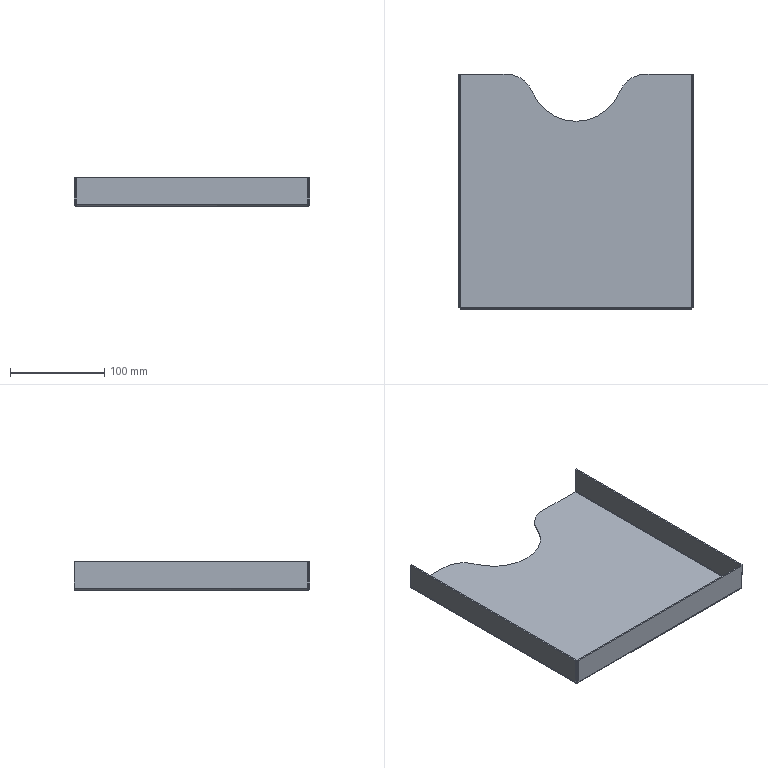Part | SolidWorks | features EdgeFlange 1, Fillet 1, FlatPattern 1, ICE 1, SMBaseFlange 1, SheetMetal 1 | 1 solid | 34 faces | box 250 x 250 x 30 mm | volume 118526 mm3 | plane 21 | cylinder 9 | spline 4 | commonest cylinder face diameters 1.473 x3 4.473 x3 60 x2 100 x1
STEP:
#1=CARTESIAN_POINT('',(122.763,125.,-1.5));
#2=VERTEX_POINT('',#1);
#3=CARTESIAN_POINT('',(74.162,125.,-1.5));
#4=VERTEX_POINT('',#3);
#5=CARTESIAN_POINT('',(-125.,125.,-1.5));
#6=DIRECTION('',(-1.,0.,0.));
#7=VECTOR('',#6,1000.);
#8=LINE('',#5,#7);
#9=EDGE_CURVE('',#2,#4,#8,.T.);
#10=ORIENTED_EDGE('',*,*,#9,.T.);
#11=CARTESIAN_POINT('',(74.162,125.,0.));
#12=VERTEX_POINT('',#11);
#13=CARTESIAN_POINT('',(74.162,125.,0.));
#14=DIRECTION('',(0.,0.,1.));
#15=VECTOR('',#14,1000.);
#16=LINE('',#13,#15);
#17=EDGE_CURVE('',#4,#12,#16,.T.);
#18=ORIENTED_EDGE('',*,*,#17,.T.);
#19=CARTESIAN_POINT('',(122.763,125.,0.));
#20=VERTEX_POINT('',#19);
#21=CARTESIAN_POINT('',(-125.,125.,0.));
#22=DIRECTION('',(-1.,0.,0.));
#23=VECTOR('',#22,1000.);
#24=LINE('',#21,#23);
#25=EDGE_CURVE('',#20,#12,#24,.T.);
#26=ORIENTED_EDGE('',*,*,#25,.F.);
#27=CARTESIAN_POINT('',(122.763,125.,0.));
#28=DIRECTION('',(0.,0.,-1.));
#29=VECTOR('',#28,1000.);
#30=LINE('',#27,#29);
#31=EDGE_CURVE('',#20,#2,#30,.T.);
#32=ORIENTED_EDGE('',*,*,#31,.T.);
#33=EDGE_LOOP('',(#10,#18,#26,#32));
#34=FACE_OUTER_BOUND('',#33,.T.);
#35=CARTESIAN_POINT('',(-125.,125.,-1.5));
#36=DIRECTION('',(0.,1.,0.));
#37=DIRECTION('',(0.,0.,1.));
#38=AXIS2_PLACEMENT_3D('',#35,#36,#37);
#39=PLANE('',#38);
#40=ADVANCED_FACE('',(#34),#39,.T.);
#41=CARTESIAN_POINT('',(-74.162,125.,-1.5));
#42=VERTEX_POINT('',#41);
#43=CARTESIAN_POINT('',(-122.763,125.,-1.5));
#44=VERTEX_POINT('',#43);
#45=CARTESIAN_POINT('',(-125.,125.,-1.5));
#46=DIRECTION('',(-1.,0.,0.));
#47=VECTOR('',#46,1000.);
#48=LINE('',#45,#47);
#49=EDGE_CURVE('',#42,#44,#48,.T.);
#50=ORIENTED_EDGE('',*,*,#49,.F.);
#51=CARTESIAN_POINT('',(-46.351,106.25,-1.5));
#52=VERTEX_POINT('',#51);
#53=CARTESIAN_POINT('',(-74.162,95.,-1.5));
#54=DIRECTION('',(0.,0.,-1.));
#55=DIRECTION('',(1.,0.,0.));
#56=AXIS2_PLACEMENT_3D('',#53,#54,#55);
#57=CIRCLE('',#56,30.);
#58=EDGE_CURVE('',#42,#52,#57,.T.);
#59=ORIENTED_EDGE('',*,*,#58,.T.);
#60=CARTESIAN_POINT('',(46.351,106.25,-1.5));
#61=VERTEX_POINT('',#60);
#62=CARTESIAN_POINT('',(0.,125.,-1.5));
#63=DIRECTION('',(0.,0.,-1.));
#64=DIRECTION('',(-1.,0.,0.));
#65=AXIS2_PLACEMENT_3D('',#62,#63,#64);
#66=CIRCLE('',#65,50.);
#67=EDGE_CURVE('',#61,#52,#66,.T.);
#68=ORIENTED_EDGE('',*,*,#67,.F.);
#69=CARTESIAN_POINT('',(74.162,95.,-1.5));
#70=DIRECTION('',(0.,0.,-1.));
#71=DIRECTION('',(1.,0.,0.));
#72=AXIS2_PLACEMENT_3D('',#69,#70,#71);
#73=CIRCLE('',#72,30.);
#74=EDGE_CURVE('',#61,#4,#73,.T.);
#75=ORIENTED_EDGE('',*,*,#74,.T.);
#76=ORIENTED_EDGE('',*,*,#9,.F.);
#77=CARTESIAN_POINT('',(122.763,-122.763,-1.5));
#78=VERTEX_POINT('',#77);
#79=CARTESIAN_POINT('',(122.763,125.,-1.5));
#80=DIRECTION('',(0.,-1.,0.));
#81=VECTOR('',#80,1000.);
#82=LINE('',#79,#81);
#83=EDGE_CURVE('',#2,#78,#82,.T.);
#84=ORIENTED_EDGE('',*,*,#83,.T.);
#85=CARTESIAN_POINT('',(-122.763,-122.763,-1.5));
#86=VERTEX_POINT('',#85);
#87=CARTESIAN_POINT('',(122.793,-122.763,-1.5));
#88=DIRECTION('',(-1.,0.,0.));
#89=VECTOR('',#88,1000.);
#90=LINE('',#87,#89);
#91=EDGE_CURVE('',#78,#86,#90,.T.);
#92=ORIENTED_EDGE('',*,*,#91,.T.);
#93=CARTESIAN_POINT('',(-122.763,-122.793,-1.5));
#94=DIRECTION('',(0.,1.,0.));
#95=VECTOR('',#94,1000.);
#96=LINE('',#93,#95);
#97=EDGE_CURVE('',#86,#44,#96,.T.);
#98=ORIENTED_EDGE('',*,*,#97,.T.);
#99=EDGE_LOOP('',(#50,#59,#68,#75,#76,#84,#92,#98));
#100=FACE_OUTER_BOUND('',#99,.T.);
#101=CARTESIAN_POINT('',(0.,0.,-1.5));
#102=DIRECTION('',(0.,0.,1.));
#103=DIRECTION('',(1.,0.,0.));
#104=AXIS2_PLACEMENT_3D('',#101,#102,#103);
#105=PLANE('',#104);
#106=ADVANCED_FACE('',(#100),#105,.F.);
#107=CARTESIAN_POINT('',(-46.351,106.25,0.));
#108=VERTEX_POINT('',#107);
#109=CARTESIAN_POINT('',(46.351,106.25,0.));
#110=VERTEX_POINT('',#109);
#111=CARTESIAN_POINT('',(0.,125.,0.));
#112=DIRECTION('',(0.,0.,1.));
#113=DIRECTION('',(1.,0.,0.));
#114=AXIS2_PLACEMENT_3D('',#111,#112,#113);
#115=CIRCLE('',#114,50.);
#116=EDGE_CURVE('',#108,#110,#115,.T.);
#117=ORIENTED_EDGE('',*,*,#116,.F.);
#118=CARTESIAN_POINT('',(-74.162,125.,0.));
#119=VERTEX_POINT('',#118);
#120=CARTESIAN_POINT('',(-74.162,95.,0.));
#121=DIRECTION('',(0.,0.,1.));
#122=DIRECTION('',(1.,0.,0.));
#123=AXIS2_PLACEMENT_3D('',#120,#121,#122);
#124=CIRCLE('',#123,30.);
#125=EDGE_CURVE('',#108,#119,#124,.T.);
#126=ORIENTED_EDGE('',*,*,#125,.T.);
#127=CARTESIAN_POINT('',(-122.763,125.,0.));
#128=VERTEX_POINT('',#127);
#129=CARTESIAN_POINT('',(-125.,125.,0.));
#130=DIRECTION('',(-1.,0.,0.));
#131=VECTOR('',#130,1000.);
#132=LINE('',#129,#131);
#133=EDGE_CURVE('',#119,#128,#132,.T.);
#134=ORIENTED_EDGE('',*,*,#133,.T.);
#135=CARTESIAN_POINT('',(-122.763,-122.763,0.));
#136=VERTEX_POINT('',#135);
#137=CARTESIAN_POINT('',(-122.763,-122.793,0.));
#138=DIRECTION('',(0.,1.,0.));
#139=VECTOR('',#138,1000.);
#140=LINE('',#137,#139);
#141=EDGE_CURVE('',#136,#128,#140,.T.);
#142=ORIENTED_EDGE('',*,*,#141,.F.);
#143=CARTESIAN_POINT('',(122.763,-122.763,0.));
#144=VERTEX_POINT('',#143);
#145=CARTESIAN_POINT('',(122.793,-122.763,0.));
#146=DIRECTION('',(-1.,0.,0.));
#147=VECTOR('',#146,1000.);
#148=LINE('',#145,#147);
#149=EDGE_CURVE('',#144,#136,#148,.T.);
#150=ORIENTED_EDGE('',*,*,#149,.F.);
#151=CARTESIAN_POINT('',(122.763,125.,0.));
#152=DIRECTION('',(0.,-1.,0.));
#153=VECTOR('',#152,1000.);
#154=LINE('',#151,#153);
#155=EDGE_CURVE('',#20,#144,#154,.T.);
#156=ORIENTED_EDGE('',*,*,#155,.F.);
#157=ORIENTED_EDGE('',*,*,#25,.T.);
#158=CARTESIAN_POINT('',(74.162,95.,0.));
#159=DIRECTION('',(0.,0.,1.));
#160=DIRECTION('',(1.,0.,0.));
#161=AXIS2_PLACEMENT_3D('',#158,#159,#160);
#162=CIRCLE('',#161,30.);
#163=EDGE_CURVE('',#12,#110,#162,.T.);
#164=ORIENTED_EDGE('',*,*,#163,.T.);
#165=EDGE_LOOP('',(#117,#126,#134,#142,#150,#156,#157,#164));
#166=FACE_OUTER_BOUND('',#165,.T.);
#167=CARTESIAN_POINT('',(0.,0.,0.));
#168=DIRECTION('',(0.,0.,1.));
#169=DIRECTION('',(1.,0.,0.));
#170=AXIS2_PLACEMENT_3D('',#167,#168,#169);
#171=PLANE('',#170);
#172=ADVANCED_FACE('',(#166),#171,.T.);
#173=ORIENTED_EDGE('',*,*,#133,.F.);
#174=CARTESIAN_POINT('',(-74.162,125.,-1.5));
#175=DIRECTION('',(0.,0.,-1.));
#176=VECTOR('',#175,1000.);
#177=LINE('',#174,#176);
#178=EDGE_CURVE('',#119,#42,#177,.T.);
#179=ORIENTED_EDGE('',*,*,#178,.T.);
#180=ORIENTED_EDGE('',*,*,#49,.T.);
#181=CARTESIAN_POINT('',(-122.763,125.,0.));
#182=DIRECTION('',(0.,0.,-1.));
#183=VECTOR('',#182,1000.);
#184=LINE('',#181,#183);
#185=EDGE_CURVE('',#128,#44,#184,.T.);
#186=ORIENTED_EDGE('',*,*,#185,.F.);
#187=EDGE_LOOP('',(#173,#179,#180,#186));
#188=FACE_OUTER_BOUND('',#187,.T.);
#189=CARTESIAN_POINT('',(-125.,125.,-1.5));
#190=DIRECTION('',(0.,1.,0.));
#191=DIRECTION('',(0.,0.,1.));
#192=AXIS2_PLACEMENT_3D('',#189,#190,#191);
#193=PLANE('',#192);
#194=ADVANCED_FACE('',(#188),#193,.T.);
#195=CARTESIAN_POINT('',(-123.5,125.,0.7366));
#196=VERTEX_POINT('',#195);
#197=CARTESIAN_POINT('',(-125.,125.,0.7366));
#198=VERTEX_POINT('',#197);
#199=CARTESIAN_POINT('',(-125.,125.,0.7366));
#200=DIRECTION('',(-1.,0.,0.));
#201=VECTOR('',#200,1000.);
#202=LINE('',#199,#201);
#203=EDGE_CURVE('',#196,#198,#202,.T.);
#204=ORIENTED_EDGE('',*,*,#203,.F.);
#205=CARTESIAN_POINT('',(-122.763,125.,0.7366));
#206=DIRECTION('',(0.,1.,0.));
#207=DIRECTION('',(0.,0.,-1.));
#208=AXIS2_PLACEMENT_3D('',#205,#206,#207);
#209=CIRCLE('',#208,0.7366);
#210=EDGE_CURVE('',#128,#196,#209,.T.);
#211=ORIENTED_EDGE('',*,*,#210,.F.);
#212=ORIENTED_EDGE('',*,*,#185,.T.);
#213=CARTESIAN_POINT('',(-122.763,125.,0.7366));
#214=DIRECTION('',(0.,1.,0.));
#215=DIRECTION('',(0.,0.,-1.));
#216=AXIS2_PLACEMENT_3D('',#213,#214,#215);
#217=CIRCLE('',#216,2.237);
#218=EDGE_CURVE('',#44,#198,#217,.T.);
#219=ORIENTED_EDGE('',*,*,#218,.T.);
#220=EDGE_LOOP('',(#204,#211,#212,#219));
#221=FACE_OUTER_BOUND('',#220,.T.);
#222=CARTESIAN_POINT('',(-122.763,125.,0.7366));
#223=DIRECTION('',(0.,1.,0.));
#224=DIRECTION('',(0.,0.,1.));
#225=AXIS2_PLACEMENT_3D('',#222,#223,#224);
#226=PLANE('',#225);
#227=ADVANCED_FACE('',(#221),#226,.T.);
#228=CARTESIAN_POINT('',(-123.5,-122.793,0.7366));
#229=VERTEX_POINT('',#228);
#230=CARTESIAN_POINT('',(-123.5,-122.793,0.7366));
#231=CARTESIAN_POINT('',(-123.5,-122.788,0.5438));
#232=CARTESIAN_POINT('',(-123.421,-122.783,0.3521));
#233=CARTESIAN_POINT('',(-123.148,-122.773,0.07939));
#234=CARTESIAN_POINT('',(-122.956,-122.768,0.));
#235=CARTESIAN_POINT('',(-122.763,-122.763,0.));
#236=B_SPLINE_CURVE_WITH_KNOTS('',3,(#230,#231,#232,#233,#234,#235),.UNSPECIFIED.,.F.,.F.,(4,2,4),(0.,0.5,1.),.UNSPECIFIED.);
#237=EDGE_CURVE('',#229,#136,#236,.T.);
#238=ORIENTED_EDGE('',*,*,#237,.F.);
#239=CARTESIAN_POINT('',(-125.,-122.793,0.7366));
#240=VERTEX_POINT('',#239);
#241=CARTESIAN_POINT('',(-123.5,-122.793,0.7366));
#242=DIRECTION('',(1.,0.,0.));
#243=VECTOR('',#242,1000.);
#244=LINE('',#241,#243);
#245=EDGE_CURVE('',#240,#229,#244,.T.);
#246=ORIENTED_EDGE('',*,*,#245,.F.);
#247=CARTESIAN_POINT('',(-125.,-122.793,0.7366));
#248=CARTESIAN_POINT('',(-125.,-122.79,0.4438));
#249=CARTESIAN_POINT('',(-124.942,-122.788,0.1512));
#250=CARTESIAN_POINT('',(-124.718,-122.783,-0.3898));
#251=CARTESIAN_POINT('',(-124.552,-122.781,-0.6379));
#252=CARTESIAN_POINT('',(-124.138,-122.776,-1.052));
#253=CARTESIAN_POINT('',(-123.89,-122.773,-1.218));
#254=CARTESIAN_POINT('',(-123.349,-122.768,-1.442));
#255=CARTESIAN_POINT('',(-123.056,-122.766,-1.5));
#256=CARTESIAN_POINT('',(-122.763,-122.763,-1.5));
#257=B_SPLINE_CURVE_WITH_KNOTS('',3,(#247,#248,#249,#250,#251,#252,#253,#254,#255,#256),.UNSPECIFIED.,.F.,.F.,(4,2,2,2,4),(0.,0.25,0.5,0.75,1.),.UNSPECIFIED.);
#258=EDGE_CURVE('',#240,#86,#257,.T.);
#259=ORIENTED_EDGE('',*,*,#258,.T.);
#260=CARTESIAN_POINT('',(-122.763,-122.763,0.));
#261=DIRECTION('',(0.,0.,-1.));
#262=VECTOR('',#261,1000.);
#263=LINE('',#260,#262);
#264=EDGE_CURVE('',#136,#86,#263,.T.);
#265=ORIENTED_EDGE('',*,*,#264,.F.);
#266=EDGE_LOOP('',(#238,#246,#259,#265));
#267=FACE_OUTER_BOUND('',#266,.T.);
#268=CARTESIAN_POINT('',(-125.015,-122.793,0.7366));
#269=CARTESIAN_POINT('',(-125.015,-122.79,0.4418));
#270=CARTESIAN_POINT('',(-124.956,-122.788,0.1472));
#271=CARTESIAN_POINT('',(-124.731,-122.783,-0.3973));
#272=CARTESIAN_POINT('',(-124.564,-122.781,-0.6471));
#273=CARTESIAN_POINT('',(-124.147,-122.776,-1.064));
#274=CARTESIAN_POINT('',(-123.897,-122.773,-1.231));
#275=CARTESIAN_POINT('',(-123.353,-122.768,-1.456));
#276=CARTESIAN_POINT('',(-123.058,-122.766,-1.515));
#277=CARTESIAN_POINT('',(-122.763,-122.763,-1.515));
#278=CARTESIAN_POINT('',(-125.,-122.793,0.7366));
#279=CARTESIAN_POINT('',(-125.,-122.79,0.4438));
#280=CARTESIAN_POINT('',(-124.942,-122.788,0.1512));
#281=CARTESIAN_POINT('',(-124.718,-122.783,-0.3898));
#282=CARTESIAN_POINT('',(-124.552,-122.781,-0.6379));
#283=CARTESIAN_POINT('',(-124.138,-122.776,-1.052));
#284=CARTESIAN_POINT('',(-123.89,-122.773,-1.218));
#285=CARTESIAN_POINT('',(-123.349,-122.768,-1.442));
#286=CARTESIAN_POINT('',(-123.056,-122.766,-1.5));
#287=CARTESIAN_POINT('',(-122.763,-122.763,-1.5));
#288=CARTESIAN_POINT('',(-123.5,-122.793,0.7366));
#289=CARTESIAN_POINT('',(-123.5,-122.79,0.6402));
#290=CARTESIAN_POINT('',(-123.481,-122.788,0.5438));
#291=CARTESIAN_POINT('',(-123.407,-122.783,0.3656));
#292=CARTESIAN_POINT('',(-123.352,-122.781,0.2839));
#293=CARTESIAN_POINT('',(-123.216,-122.776,0.1476));
#294=CARTESIAN_POINT('',(-123.134,-122.773,0.09297));
#295=CARTESIAN_POINT('',(-122.956,-122.768,0.01917));
#296=CARTESIAN_POINT('',(-122.86,-122.766,0.));
#297=CARTESIAN_POINT('',(-122.763,-122.763,0.));
#298=CARTESIAN_POINT('',(-123.485,-122.793,0.7366));
#299=CARTESIAN_POINT('',(-123.485,-122.79,0.6421));
#300=CARTESIAN_POINT('',(-123.466,-122.788,0.5478));
#301=CARTESIAN_POINT('',(-123.394,-122.783,0.3733));
#302=CARTESIAN_POINT('',(-123.34,-122.781,0.2932));
#303=CARTESIAN_POINT('',(-123.207,-122.776,0.1597));
#304=CARTESIAN_POINT('',(-123.127,-122.773,0.1062));
#305=CARTESIAN_POINT('',(-122.952,-122.768,0.03393));
#306=CARTESIAN_POINT('',(-122.858,-122.766,0.01515));
#307=CARTESIAN_POINT('',(-122.763,-122.763,0.01515));
#308=B_SPLINE_SURFACE_WITH_KNOTS('',1,3,((#268,#269,#270,#271,#272,#273,#274,#275,#276,#277),(#278,#279,#280,#281,#282,#283,#284,#285,#286,#287),(#288,#289,#290,#291,#292,#293,#294,#295,#296,#297),(#298,#299,#300,#301,#302,#303,#304,#305,#306,#307)),.UNSPECIFIED.,.F.,.F.,.F.,(2,1,1,2),(4,2,2,2,4),(-0.01,0.,1.,1.01),(0.,0.25,0.5,0.75,1.),.UNSPECIFIED.);
#309=ADVANCED_FACE('',(#267),#308,.F.);
#310=ORIENTED_EDGE('',*,*,#97,.F.);
#311=ORIENTED_EDGE('',*,*,#258,.F.);
#312=CARTESIAN_POINT('',(-125.,125.,0.7366));
#313=DIRECTION('',(0.,1.,0.));
#314=VECTOR('',#313,1000.);
#315=LINE('',#312,#314);
#316=EDGE_CURVE('',#240,#198,#315,.T.);
#317=ORIENTED_EDGE('',*,*,#316,.T.);
#318=ORIENTED_EDGE('',*,*,#218,.F.);
#319=EDGE_LOOP('',(#310,#311,#317,#318));
#320=FACE_OUTER_BOUND('',#319,.T.);
#321=CARTESIAN_POINT('',(-122.763,-122.793,0.7366));
#322=DIRECTION('',(0.,-1.,0.));
#323=DIRECTION('',(-1.,0.,0.));
#324=AXIS2_PLACEMENT_3D('',#321,#322,#323);
#325=CYLINDRICAL_SURFACE('',#324,2.237);
#326=ADVANCED_FACE('',(#320),#325,.T.);
#327=ORIENTED_EDGE('',*,*,#141,.T.);
#328=ORIENTED_EDGE('',*,*,#210,.T.);
#329=CARTESIAN_POINT('',(-123.5,125.,0.7366));
#330=DIRECTION('',(0.,-1.,0.));
#331=VECTOR('',#330,1000.);
#332=LINE('',#329,#331);
#333=EDGE_CURVE('',#196,#229,#332,.T.);
#334=ORIENTED_EDGE('',*,*,#333,.T.);
#335=ORIENTED_EDGE('',*,*,#237,.T.);
#336=EDGE_LOOP('',(#327,#328,#334,#335));
#337=FACE_OUTER_BOUND('',#336,.T.);
#338=CARTESIAN_POINT('',(-122.763,-122.793,0.7366));
#339=DIRECTION('',(0.,-1.,0.));
#340=DIRECTION('',(-1.,0.,0.));
#341=AXIS2_PLACEMENT_3D('',#338,#339,#340);
#342=CYLINDRICAL_SURFACE('',#341,0.7366);
#343=ADVANCED_FACE('',(#337),#342,.F.);
#344=ORIENTED_EDGE('',*,*,#203,.T.);
#345=CARTESIAN_POINT('',(-125.,125.,28.5));
#346=VERTEX_POINT('',#345);
#347=CARTESIAN_POINT('',(-125.,125.,0.));
#348=DIRECTION('',(0.,0.,-1.));
#349=VECTOR('',#348,1000.);
#350=LINE('',#347,#349);
#351=EDGE_CURVE('',#346,#198,#350,.T.);
#352=ORIENTED_EDGE('',*,*,#351,.F.);
#353=CARTESIAN_POINT('',(-123.5,125.,28.5));
#354=VERTEX_POINT('',#353);
#355=CARTESIAN_POINT('',(-125.,125.,28.5));
#356=DIRECTION('',(1.,0.,0.));
#357=VECTOR('',#356,1000.);
#358=LINE('',#355,#357);
#359=EDGE_CURVE('',#346,#354,#358,.T.);
#360=ORIENTED_EDGE('',*,*,#359,.T.);
#361=CARTESIAN_POINT('',(-123.5,125.,0.));
#362=DIRECTION('',(0.,0.,-1.));
#363=VECTOR('',#362,1000.);
#364=LINE('',#361,#363);
#365=EDGE_CURVE('',#354,#196,#364,.T.);
#366=ORIENTED_EDGE('',*,*,#365,.T.);
#367=EDGE_LOOP('',(#344,#352,#360,#366));
#368=FACE_OUTER_BOUND('',#367,.T.);
#369=CARTESIAN_POINT('',(-125.,125.,0.));
#370=DIRECTION('',(0.,-1.,0.));
#371=DIRECTION('',(1.,0.,0.));
#372=AXIS2_PLACEMENT_3D('',#369,#370,#371);
#373=PLANE('',#372);
#374=ADVANCED_FACE('',(#368),#373,.F.);
#375=ORIENTED_EDGE('',*,*,#316,.F.);
#376=CARTESIAN_POINT('',(-125.,-122.793,28.5));
#377=VERTEX_POINT('',#376);
#378=CARTESIAN_POINT('',(-125.,-122.793,0.));
#379=DIRECTION('',(0.,0.,1.));
#380=VECTOR('',#379,1000.);
#381=LINE('',#378,#380);
#382=EDGE_CURVE('',#240,#377,#381,.T.);
#383=ORIENTED_EDGE('',*,*,#382,.T.);
#384=CARTESIAN_POINT('',(-125.,0.,28.5));
#385=DIRECTION('',(0.,1.,0.));
#386=VECTOR('',#385,1000.);
#387=LINE('',#384,#386);
#388=EDGE_CURVE('',#377,#346,#387,.T.);
#389=ORIENTED_EDGE('',*,*,#388,.T.);
#390=ORIENTED_EDGE('',*,*,#351,.T.);
#391=EDGE_LOOP('',(#375,#383,#389,#390));
#392=FACE_OUTER_BOUND('',#391,.T.);
#393=CARTESIAN_POINT('',(-125.,0.,0.));
#394=DIRECTION('',(1.,0.,0.));
#395=DIRECTION('',(0.,0.,-1.));
#396=AXIS2_PLACEMENT_3D('',#393,#394,#395);
#397=PLANE('',#396);
#398=ADVANCED_FACE('',(#392),#397,.F.);
#399=CARTESIAN_POINT('',(-123.5,-122.793,28.5));
#400=VERTEX_POINT('',#399);
#401=CARTESIAN_POINT('',(-123.5,-122.793,0.));
#402=DIRECTION('',(0.,0.,1.));
#403=VECTOR('',#402,1000.);
#404=LINE('',#401,#403);
#405=EDGE_CURVE('',#229,#400,#404,.T.);
#406=ORIENTED_EDGE('',*,*,#405,.F.);
#407=ORIENTED_EDGE('',*,*,#333,.F.);
#408=ORIENTED_EDGE('',*,*,#365,.F.);
#409=CARTESIAN_POINT('',(-123.5,125.,28.5));
#410=DIRECTION('',(0.,1.,0.));
#411=VECTOR('',#410,1000.);
#412=LINE('',#409,#411);
#413=EDGE_CURVE('',#400,#354,#412,.T.);
#414=ORIENTED_EDGE('',*,*,#413,.F.);
#415=EDGE_LOOP('',(#406,#407,#408,#414));
#416=FACE_OUTER_BOUND('',#415,.T.);
#417=CARTESIAN_POINT('',(-123.5,0.,0.));
#418=DIRECTION('',(1.,0.,0.));
#419=DIRECTION('',(0.,0.,-1.));
#420=AXIS2_PLACEMENT_3D('',#417,#418,#419);
#421=PLANE('',#420);
#422=ADVANCED_FACE('',(#416),#421,.T.);
#423=ORIENTED_EDGE('',*,*,#388,.F.);
#424=CARTESIAN_POINT('',(-125.,-122.793,28.5));
#425=DIRECTION('',(1.,0.,0.));
#426=VECTOR('',#425,1000.);
#427=LINE('',#424,#426);
#428=EDGE_CURVE('',#377,#400,#427,.T.);
#429=ORIENTED_EDGE('',*,*,#428,.T.);
#430=ORIENTED_EDGE('',*,*,#413,.T.);
#431=ORIENTED_EDGE('',*,*,#359,.F.);
#432=EDGE_LOOP('',(#423,#429,#430,#431));
#433=FACE_OUTER_BOUND('',#432,.T.);
#434=CARTESIAN_POINT('',(-125.,125.,28.5));
#435=DIRECTION('',(0.,0.,-1.));
#436=DIRECTION('',(-1.,0.,0.));
#437=AXIS2_PLACEMENT_3D('',#434,#435,#436);
#438=PLANE('',#437);
#439=ADVANCED_FACE('',(#433),#438,.F.);
#440=ORIENTED_EDGE('',*,*,#428,.F.);
#441=ORIENTED_EDGE('',*,*,#382,.F.);
#442=ORIENTED_EDGE('',*,*,#245,.T.);
#443=ORIENTED_EDGE('',*,*,#405,.T.);
#444=EDGE_LOOP('',(#440,#441,#442,#443));
#445=FACE_OUTER_BOUND('',#444,.T.);
#446=CARTESIAN_POINT('',(-123.5,-122.793,0.));
#447=DIRECTION('',(0.,1.,0.));
#448=DIRECTION('',(0.,0.,1.));
#449=AXIS2_PLACEMENT_3D('',#446,#447,#448);
#450=PLANE('',#449);
#451=ADVANCED_FACE('',(#445),#450,.F.);
#452=CARTESIAN_POINT('',(125.,-122.793,0.7366));
#453=VERTEX_POINT('',#452);
#454=CARTESIAN_POINT('',(123.5,-122.793,0.7366));
#455=VERTEX_POINT('',#454);
#456=CARTESIAN_POINT('',(123.5,-122.793,0.7366));
#457=DIRECTION('',(-1.,0.,0.));
#458=VECTOR('',#457,1000.);
#459=LINE('',#456,#458);
#460=EDGE_CURVE('',#453,#455,#459,.T.);
#461=ORIENTED_EDGE('',*,*,#460,.T.);
#462=CARTESIAN_POINT('',(122.763,-122.763,0.));
#463=CARTESIAN_POINT('',(122.956,-122.768,0.));
#464=CARTESIAN_POINT('',(123.148,-122.773,0.07939));
#465=CARTESIAN_POINT('',(123.421,-122.783,0.3521));
#466=CARTESIAN_POINT('',(123.5,-122.788,0.5438));
#467=CARTESIAN_POINT('',(123.5,-122.793,0.7366));
#468=B_SPLINE_CURVE_WITH_KNOTS('',3,(#462,#463,#464,#465,#466,#467),.UNSPECIFIED.,.F.,.F.,(4,2,4),(0.,0.5,1.),.UNSPECIFIED.);
#469=EDGE_CURVE('',#144,#455,#468,.T.);
#470=ORIENTED_EDGE('',*,*,#469,.F.);
#471=CARTESIAN_POINT('',(122.763,-122.763,0.));
#472=DIRECTION('',(0.,0.,-1.));
#473=VECTOR('',#472,1000.);
#474=LINE('',#471,#473);
#475=EDGE_CURVE('',#144,#78,#474,.T.);
#476=ORIENTED_EDGE('',*,*,#475,.T.);
#477=CARTESIAN_POINT('',(122.763,-122.763,-1.5));
#478=CARTESIAN_POINT('',(123.056,-122.766,-1.5));
#479=CARTESIAN_POINT('',(123.349,-122.768,-1.442));
#480=CARTESIAN_POINT('',(123.89,-122.773,-1.218));
#481=CARTESIAN_POINT('',(124.138,-122.776,-1.052));
#482=CARTESIAN_POINT('',(124.552,-122.781,-0.6379));
#483=CARTESIAN_POINT('',(124.718,-122.783,-0.3898));
#484=CARTESIAN_POINT('',(124.942,-122.788,0.1512));
#485=CARTESIAN_POINT('',(125.,-122.79,0.4438));
#486=CARTESIAN_POINT('',(125.,-122.793,0.7366));
#487=B_SPLINE_CURVE_WITH_KNOTS('',3,(#477,#478,#479,#480,#481,#482,#483,#484,#485,#486),.UNSPECIFIED.,.F.,.F.,(4,2,2,2,4),(0.,0.25,0.5,0.75,1.),.UNSPECIFIED.);
#488=EDGE_CURVE('',#78,#453,#487,.T.);
#489=ORIENTED_EDGE('',*,*,#488,.T.);
#490=EDGE_LOOP('',(#461,#470,#476,#489));
#491=FACE_OUTER_BOUND('',#490,.T.);
#492=CARTESIAN_POINT('',(122.763,-122.763,-1.515));
#493=CARTESIAN_POINT('',(123.058,-122.766,-1.515));
#494=CARTESIAN_POINT('',(123.353,-122.768,-1.456));
#495=CARTESIAN_POINT('',(123.897,-122.773,-1.231));
#496=CARTESIAN_POINT('',(124.147,-122.776,-1.064));
#497=CARTESIAN_POINT('',(124.564,-122.781,-0.6471));
#498=CARTESIAN_POINT('',(124.731,-122.783,-0.3973));
#499=CARTESIAN_POINT('',(124.956,-122.788,0.1472));
#500=CARTESIAN_POINT('',(125.015,-122.79,0.4418));
#501=CARTESIAN_POINT('',(125.015,-122.793,0.7366));
#502=CARTESIAN_POINT('',(122.763,-122.763,-1.5));
#503=CARTESIAN_POINT('',(123.056,-122.766,-1.5));
#504=CARTESIAN_POINT('',(123.349,-122.768,-1.442));
#505=CARTESIAN_POINT('',(123.89,-122.773,-1.218));
#506=CARTESIAN_POINT('',(124.138,-122.776,-1.052));
#507=CARTESIAN_POINT('',(124.552,-122.781,-0.6379));
#508=CARTESIAN_POINT('',(124.718,-122.783,-0.3898));
#509=CARTESIAN_POINT('',(124.942,-122.788,0.1512));
#510=CARTESIAN_POINT('',(125.,-122.79,0.4438));
#511=CARTESIAN_POINT('',(125.,-122.793,0.7366));
#512=CARTESIAN_POINT('',(122.763,-122.763,0.));
#513=CARTESIAN_POINT('',(122.86,-122.766,0.));
#514=CARTESIAN_POINT('',(122.956,-122.768,0.01917));
#515=CARTESIAN_POINT('',(123.134,-122.773,0.09297));
#516=CARTESIAN_POINT('',(123.216,-122.776,0.1476));
#517=CARTESIAN_POINT('',(123.352,-122.781,0.2839));
#518=CARTESIAN_POINT('',(123.407,-122.783,0.3656));
#519=CARTESIAN_POINT('',(123.481,-122.788,0.5438));
#520=CARTESIAN_POINT('',(123.5,-122.79,0.6402));
#521=CARTESIAN_POINT('',(123.5,-122.793,0.7366));
#522=CARTESIAN_POINT('',(122.763,-122.763,0.01515));
#523=CARTESIAN_POINT('',(122.858,-122.766,0.01515));
#524=CARTESIAN_POINT('',(122.952,-122.768,0.03393));
#525=CARTESIAN_POINT('',(123.127,-122.773,0.1062));
#526=CARTESIAN_POINT('',(123.207,-122.776,0.1597));
#527=CARTESIAN_POINT('',(123.34,-122.781,0.2932));
#528=CARTESIAN_POINT('',(123.394,-122.783,0.3733));
#529=CARTESIAN_POINT('',(123.466,-122.788,0.5478));
#530=CARTESIAN_POINT('',(123.485,-122.79,0.6421));
#531=CARTESIAN_POINT('',(123.485,-122.793,0.7366));
#532=B_SPLINE_SURFACE_WITH_KNOTS('',1,3,((#492,#493,#494,#495,#496,#497,#498,#499,#500,#501),(#502,#503,#504,#505,#506,#507,#508,#509,#510,#511),(#512,#513,#514,#515,#516,#517,#518,#519,#520,#521),(#522,#523,#524,#525,#526,#527,#528,#529,#530,#531)),.UNSPECIFIED.,.F.,.F.,.F.,(2,1,1,2),(4,2,2,2,4),(-0.01,0.,1.,1.01),(0.,0.25,0.5,0.75,1.),.UNSPECIFIED.);
#533=ADVANCED_FACE('',(#491),#532,.F.);
#534=CARTESIAN_POINT('',(123.5,125.,0.7366));
#535=VERTEX_POINT('',#534);
#536=CARTESIAN_POINT('',(122.763,125.,0.7366));
#537=DIRECTION('',(0.,1.,0.));
#538=DIRECTION('',(0.,0.,1.));
#539=AXIS2_PLACEMENT_3D('',#536,#537,#538);
#540=CIRCLE('',#539,0.7366);
#541=EDGE_CURVE('',#535,#20,#540,.T.);
#542=ORIENTED_EDGE('',*,*,#541,.F.);
#543=CARTESIAN_POINT('',(125.,125.,0.7366));
#544=VERTEX_POINT('',#543);
#545=CARTESIAN_POINT('',(123.5,125.,0.7366));
#546=DIRECTION('',(1.,0.,0.));
#547=VECTOR('',#546,1000.);
#548=LINE('',#545,#547);
#549=EDGE_CURVE('',#535,#544,#548,.T.);
#550=ORIENTED_EDGE('',*,*,#549,.T.);
#551=CARTESIAN_POINT('',(122.763,125.,0.7366));
#552=DIRECTION('',(0.,1.,0.));
#553=DIRECTION('',(0.,0.,1.));
#554=AXIS2_PLACEMENT_3D('',#551,#552,#553);
#555=CIRCLE('',#554,2.237);
#556=EDGE_CURVE('',#544,#2,#555,.T.);
#557=ORIENTED_EDGE('',*,*,#556,.T.);
#558=ORIENTED_EDGE('',*,*,#31,.F.);
#559=EDGE_LOOP('',(#542,#550,#557,#558));
#560=FACE_OUTER_BOUND('',#559,.T.);
#561=CARTESIAN_POINT('',(122.763,125.,0.7366));
#562=DIRECTION('',(0.,-1.,0.));
#563=DIRECTION('',(0.,0.,-1.));
#564=AXIS2_PLACEMENT_3D('',#561,#562,#563);
#565=PLANE('',#564);
#566=ADVANCED_FACE('',(#560),#565,.F.);
#567=ORIENTED_EDGE('',*,*,#83,.F.);
#568=ORIENTED_EDGE('',*,*,#556,.F.);
#569=CARTESIAN_POINT('',(125.,-125.,0.7366));
#570=DIRECTION('',(0.,-1.,0.));
#571=VECTOR('',#570,1000.);
#572=LINE('',#569,#571);
#573=EDGE_CURVE('',#544,#453,#572,.T.);
#574=ORIENTED_EDGE('',*,*,#573,.T.);
#575=ORIENTED_EDGE('',*,*,#488,.F.);
#576=EDGE_LOOP('',(#567,#568,#574,#575));
#577=FACE_OUTER_BOUND('',#576,.T.);
#578=CARTESIAN_POINT('',(122.763,125.,0.7366));
#579=DIRECTION('',(0.,1.,0.));
#580=DIRECTION('',(1.,0.,0.));
#581=AXIS2_PLACEMENT_3D('',#578,#579,#580);
#582=CYLINDRICAL_SURFACE('',#581,2.237);
#583=ADVANCED_FACE('',(#577),#582,.T.);
#584=ORIENTED_EDGE('',*,*,#155,.T.);
#585=ORIENTED_EDGE('',*,*,#469,.T.);
#586=CARTESIAN_POINT('',(123.5,-125.,0.7366));
#587=DIRECTION('',(0.,1.,0.));
#588=VECTOR('',#587,1000.);
#589=LINE('',#586,#588);
#590=EDGE_CURVE('',#455,#535,#589,.T.);
#591=ORIENTED_EDGE('',*,*,#590,.T.);
#592=ORIENTED_EDGE('',*,*,#541,.T.);
#593=EDGE_LOOP('',(#584,#585,#591,#592));
#594=FACE_OUTER_BOUND('',#593,.T.);
#595=CARTESIAN_POINT('',(122.763,125.,0.7366));
#596=DIRECTION('',(0.,1.,0.));
#597=DIRECTION('',(1.,0.,0.));
#598=AXIS2_PLACEMENT_3D('',#595,#596,#597);
#599=CYLINDRICAL_SURFACE('',#598,0.7366);
#600=ADVANCED_FACE('',(#594),#599,.F.);
#601=CARTESIAN_POINT('',(125.,-122.793,28.5));
#602=VERTEX_POINT('',#601);
#603=CARTESIAN_POINT('',(125.,-122.793,0.));
#604=DIRECTION('',(0.,0.,1.));
#605=VECTOR('',#604,1000.);
#606=LINE('',#603,#605);
#607=EDGE_CURVE('',#453,#602,#606,.T.);
#608=ORIENTED_EDGE('',*,*,#607,.T.);
#609=CARTESIAN_POINT('',(123.5,-122.793,28.5));
#610=VERTEX_POINT('',#609);
#611=CARTESIAN_POINT('',(123.5,-122.793,28.5));
#612=DIRECTION('',(-1.,0.,0.));
#613=VECTOR('',#612,1000.);
#614=LINE('',#611,#613);
#615=EDGE_CURVE('',#602,#610,#614,.T.);
#616=ORIENTED_EDGE('',*,*,#615,.T.);
#617=CARTESIAN_POINT('',(123.5,-122.793,0.));
#618=DIRECTION('',(0.,0.,1.));
#619=VECTOR('',#618,1000.);
#620=LINE('',#617,#619);
#621=EDGE_CURVE('',#455,#610,#620,.T.);
#622=ORIENTED_EDGE('',*,*,#621,.F.);
#623=ORIENTED_EDGE('',*,*,#460,.F.);
#624=EDGE_LOOP('',(#608,#616,#622,#623));
#625=FACE_OUTER_BOUND('',#624,.T.);
#626=CARTESIAN_POINT('',(123.5,-122.793,0.));
#627=DIRECTION('',(0.,-1.,0.));
#628=DIRECTION('',(0.,0.,-1.));
#629=AXIS2_PLACEMENT_3D('',#626,#627,#628);
#630=PLANE('',#629);
#631=ADVANCED_FACE('',(#625),#630,.T.);
#632=ORIENTED_EDGE('',*,*,#607,.F.);
#633=ORIENTED_EDGE('',*,*,#573,.F.);
#634=CARTESIAN_POINT('',(125.,125.,28.5));
#635=VERTEX_POINT('',#634);
#636=CARTESIAN_POINT('',(125.,125.,0.));
#637=DIRECTION('',(0.,0.,1.));
#638=VECTOR('',#637,1000.);
#639=LINE('',#636,#638);
#640=EDGE_CURVE('',#544,#635,#639,.T.);
#641=ORIENTED_EDGE('',*,*,#640,.T.);
#642=CARTESIAN_POINT('',(125.,0.,28.5));
#643=DIRECTION('',(0.,-1.,0.));
#644=VECTOR('',#643,1000.);
#645=LINE('',#642,#644);
#646=EDGE_CURVE('',#635,#602,#645,.T.);
#647=ORIENTED_EDGE('',*,*,#646,.T.);
#648=EDGE_LOOP('',(#632,#633,#641,#647));
#649=FACE_OUTER_BOUND('',#648,.T.);
#650=CARTESIAN_POINT('',(125.,0.,0.));
#651=DIRECTION('',(-1.,0.,0.));
#652=DIRECTION('',(0.,0.,1.));
#653=AXIS2_PLACEMENT_3D('',#650,#651,#652);
#654=PLANE('',#653);
#655=ADVANCED_FACE('',(#649),#654,.F.);
#656=ORIENTED_EDGE('',*,*,#590,.F.);
#657=ORIENTED_EDGE('',*,*,#621,.T.);
#658=CARTESIAN_POINT('',(123.5,125.,28.5));
#659=VERTEX_POINT('',#658);
#660=CARTESIAN_POINT('',(123.5,-125.,28.5));
#661=DIRECTION('',(0.,-1.,0.));
#662=VECTOR('',#661,1000.);
#663=LINE('',#660,#662);
#664=EDGE_CURVE('',#659,#610,#663,.T.);
#665=ORIENTED_EDGE('',*,*,#664,.F.);
#666=CARTESIAN_POINT('',(123.5,125.,28.5));
#667=DIRECTION('',(0.,0.,1.));
#668=VECTOR('',#667,1000.);
#669=LINE('',#666,#668);
#670=EDGE_CURVE('',#535,#659,#669,.T.);
#671=ORIENTED_EDGE('',*,*,#670,.F.);
#672=EDGE_LOOP('',(#656,#657,#665,#671));
#673=FACE_OUTER_BOUND('',#672,.T.);
#674=CARTESIAN_POINT('',(123.5,0.,0.));
#675=DIRECTION('',(-1.,0.,0.));
#676=DIRECTION('',(0.,0.,1.));
#677=AXIS2_PLACEMENT_3D('',#674,#675,#676);
#678=PLANE('',#677);
#679=ADVANCED_FACE('',(#673),#678,.T.);
#680=ORIENTED_EDGE('',*,*,#615,.F.);
#681=ORIENTED_EDGE('',*,*,#646,.F.);
#682=CARTESIAN_POINT('',(125.,125.,28.5));
#683=DIRECTION('',(-1.,0.,0.));
#684=VECTOR('',#683,1000.);
#685=LINE('',#682,#684);
#686=EDGE_CURVE('',#635,#659,#685,.T.);
#687=ORIENTED_EDGE('',*,*,#686,.T.);
#688=ORIENTED_EDGE('',*,*,#664,.T.);
#689=EDGE_LOOP('',(#680,#681,#687,#688));
#690=FACE_OUTER_BOUND('',#689,.T.);
#691=CARTESIAN_POINT('',(125.,-125.,28.5));
#692=DIRECTION('',(0.,0.,-1.));
#693=DIRECTION('',(-1.,0.,0.));
#694=AXIS2_PLACEMENT_3D('',#691,#692,#693);
#695=PLANE('',#694);
#696=ADVANCED_FACE('',(#690),#695,.F.);
#697=ORIENTED_EDGE('',*,*,#549,.F.);
#698=ORIENTED_EDGE('',*,*,#670,.T.);
#699=ORIENTED_EDGE('',*,*,#686,.F.);
#700=ORIENTED_EDGE('',*,*,#640,.F.);
#701=EDGE_LOOP('',(#697,#698,#699,#700));
#702=FACE_OUTER_BOUND('',#701,.T.);
#703=CARTESIAN_POINT('',(125.,125.,28.5));
#704=DIRECTION('',(0.,-1.,0.));
#705=DIRECTION('',(1.,0.,0.));
#706=AXIS2_PLACEMENT_3D('',#703,#704,#705);
#707=PLANE('',#706);
#708=ADVANCED_FACE('',(#702),#707,.F.);
#709=CARTESIAN_POINT('',(-122.793,-125.,0.7366));
#710=VERTEX_POINT('',#709);
#711=CARTESIAN_POINT('',(-122.793,-123.5,0.7366));
#712=VERTEX_POINT('',#711);
#713=CARTESIAN_POINT('',(-122.793,-123.5,0.7366));
#714=DIRECTION('',(0.,1.,0.));
#715=VECTOR('',#714,1000.);
#716=LINE('',#713,#715);
#717=EDGE_CURVE('',#710,#712,#716,.T.);
#718=ORIENTED_EDGE('',*,*,#717,.T.);
#719=CARTESIAN_POINT('',(-122.763,-122.763,0.));
#720=CARTESIAN_POINT('',(-122.768,-122.956,0.));
#721=CARTESIAN_POINT('',(-122.773,-123.148,0.07939));
#722=CARTESIAN_POINT('',(-122.783,-123.421,0.3521));
#723=CARTESIAN_POINT('',(-122.788,-123.5,0.5438));
#724=CARTESIAN_POINT('',(-122.793,-123.5,0.7366));
#725=B_SPLINE_CURVE_WITH_KNOTS('',3,(#719,#720,#721,#722,#723,#724),.UNSPECIFIED.,.F.,.F.,(4,2,4),(0.,0.5,1.),.UNSPECIFIED.);
#726=EDGE_CURVE('',#136,#712,#725,.T.);
#727=ORIENTED_EDGE('',*,*,#726,.F.);
#728=ORIENTED_EDGE('',*,*,#264,.T.);
#729=CARTESIAN_POINT('',(-122.763,-122.763,-1.5));
#730=CARTESIAN_POINT('',(-122.766,-123.056,-1.5));
#731=CARTESIAN_POINT('',(-122.768,-123.349,-1.442));
#732=CARTESIAN_POINT('',(-122.773,-123.89,-1.218));
#733=CARTESIAN_POINT('',(-122.776,-124.138,-1.052));
#734=CARTESIAN_POINT('',(-122.781,-124.552,-0.6379));
#735=CARTESIAN_POINT('',(-122.783,-124.718,-0.3898));
#736=CARTESIAN_POINT('',(-122.788,-124.942,0.1512));
#737=CARTESIAN_POINT('',(-122.79,-125.,0.4438));
#738=CARTESIAN_POINT('',(-122.793,-125.,0.7366));
#739=B_SPLINE_CURVE_WITH_KNOTS('',3,(#729,#730,#731,#732,#733,#734,#735,#736,#737,#738),.UNSPECIFIED.,.F.,.F.,(4,2,2,2,4),(0.,0.25,0.5,0.75,1.),.UNSPECIFIED.);
#740=EDGE_CURVE('',#86,#710,#739,.T.);
#741=ORIENTED_EDGE('',*,*,#740,.T.);
#742=EDGE_LOOP('',(#718,#727,#728,#741));
#743=FACE_OUTER_BOUND('',#742,.T.);
#744=CARTESIAN_POINT('',(-122.763,-122.763,-1.515));
#745=CARTESIAN_POINT('',(-122.766,-123.058,-1.515));
#746=CARTESIAN_POINT('',(-122.768,-123.353,-1.456));
#747=CARTESIAN_POINT('',(-122.773,-123.897,-1.231));
#748=CARTESIAN_POINT('',(-122.776,-124.147,-1.064));
#749=CARTESIAN_POINT('',(-122.781,-124.564,-0.6471));
#750=CARTESIAN_POINT('',(-122.783,-124.731,-0.3973));
#751=CARTESIAN_POINT('',(-122.788,-124.956,0.1472));
#752=CARTESIAN_POINT('',(-122.79,-125.015,0.4418));
#753=CARTESIAN_POINT('',(-122.793,-125.015,0.7366));
#754=CARTESIAN_POINT('',(-122.763,-122.763,-1.5));
#755=CARTESIAN_POINT('',(-122.766,-123.056,-1.5));
#756=CARTESIAN_POINT('',(-122.768,-123.349,-1.442));
#757=CARTESIAN_POINT('',(-122.773,-123.89,-1.218));
#758=CARTESIAN_POINT('',(-122.776,-124.138,-1.052));
#759=CARTESIAN_POINT('',(-122.781,-124.552,-0.6379));
#760=CARTESIAN_POINT('',(-122.783,-124.718,-0.3898));
#761=CARTESIAN_POINT('',(-122.788,-124.942,0.1512));
#762=CARTESIAN_POINT('',(-122.79,-125.,0.4438));
#763=CARTESIAN_POINT('',(-122.793,-125.,0.7366));
#764=CARTESIAN_POINT('',(-122.763,-122.763,0.));
#765=CARTESIAN_POINT('',(-122.766,-122.86,0.));
#766=CARTESIAN_POINT('',(-122.768,-122.956,0.01917));
#767=CARTESIAN_POINT('',(-122.773,-123.134,0.09297));
#768=CARTESIAN_POINT('',(-122.776,-123.216,0.1476));
#769=CARTESIAN_POINT('',(-122.781,-123.352,0.2839));
#770=CARTESIAN_POINT('',(-122.783,-123.407,0.3656));
#771=CARTESIAN_POINT('',(-122.788,-123.481,0.5438));
#772=CARTESIAN_POINT('',(-122.79,-123.5,0.6402));
#773=CARTESIAN_POINT('',(-122.793,-123.5,0.7366));
#774=CARTESIAN_POINT('',(-122.763,-122.763,0.01515));
#775=CARTESIAN_POINT('',(-122.766,-122.858,0.01515));
#776=CARTESIAN_POINT('',(-122.768,-122.952,0.03393));
#777=CARTESIAN_POINT('',(-122.773,-123.127,0.1062));
#778=CARTESIAN_POINT('',(-122.776,-123.207,0.1597));
#779=CARTESIAN_POINT('',(-122.781,-123.34,0.2932));
#780=CARTESIAN_POINT('',(-122.783,-123.394,0.3733));
#781=CARTESIAN_POINT('',(-122.788,-123.466,0.5478));
#782=CARTESIAN_POINT('',(-122.79,-123.485,0.6421));
#783=CARTESIAN_POINT('',(-122.793,-123.485,0.7366));
#784=B_SPLINE_SURFACE_WITH_KNOTS('',1,3,((#744,#745,#746,#747,#748,#749,#750,#751,#752,#753),(#754,#755,#756,#757,#758,#759,#760,#761,#762,#763),(#764,#765,#766,#767,#768,#769,#770,#771,#772,#773),(#774,#775,#776,#777,#778,#779,#780,#781,#782,#783)),.UNSPECIFIED.,.F.,.F.,.F.,(2,1,1,2),(4,2,2,2,4),(-0.01,0.,1.,1.01),(0.,0.25,0.5,0.75,1.),.UNSPECIFIED.);
#785=ADVANCED_FACE('',(#743),#784,.F.);
#786=CARTESIAN_POINT('',(122.793,-123.5,0.7366));
#787=VERTEX_POINT('',#786);
#788=CARTESIAN_POINT('',(122.793,-123.5,0.7366));
#789=CARTESIAN_POINT('',(122.788,-123.5,0.5438));
#790=CARTESIAN_POINT('',(122.783,-123.421,0.3521));
#791=CARTESIAN_POINT('',(122.773,-123.148,0.07939));
#792=CARTESIAN_POINT('',(122.768,-122.956,0.));
#793=CARTESIAN_POINT('',(122.763,-122.763,0.));
#794=B_SPLINE_CURVE_WITH_KNOTS('',3,(#788,#789,#790,#791,#792,#793),.UNSPECIFIED.,.F.,.F.,(4,2,4),(0.,0.5,1.),.UNSPECIFIED.);
#795=EDGE_CURVE('',#787,#144,#794,.T.);
#796=ORIENTED_EDGE('',*,*,#795,.F.);
#797=CARTESIAN_POINT('',(122.793,-125.,0.7366));
#798=VERTEX_POINT('',#797);
#799=CARTESIAN_POINT('',(122.793,-123.5,0.7366));
#800=DIRECTION('',(0.,1.,0.));
#801=VECTOR('',#800,1000.);
#802=LINE('',#799,#801);
#803=EDGE_CURVE('',#798,#787,#802,.T.);
#804=ORIENTED_EDGE('',*,*,#803,.F.);
#805=CARTESIAN_POINT('',(122.793,-125.,0.7366));
#806=CARTESIAN_POINT('',(122.79,-125.,0.4438));
#807=CARTESIAN_POINT('',(122.788,-124.942,0.1512));
#808=CARTESIAN_POINT('',(122.783,-124.718,-0.3898));
#809=CARTESIAN_POINT('',(122.781,-124.552,-0.6379));
#810=CARTESIAN_POINT('',(122.776,-124.138,-1.052));
#811=CARTESIAN_POINT('',(122.773,-123.89,-1.218));
#812=CARTESIAN_POINT('',(122.768,-123.349,-1.442));
#813=CARTESIAN_POINT('',(122.766,-123.056,-1.5));
#814=CARTESIAN_POINT('',(122.763,-122.763,-1.5));
#815=B_SPLINE_CURVE_WITH_KNOTS('',3,(#805,#806,#807,#808,#809,#810,#811,#812,#813,#814),.UNSPECIFIED.,.F.,.F.,(4,2,2,2,4),(0.,0.25,0.5,0.75,1.),.UNSPECIFIED.);
#816=EDGE_CURVE('',#798,#78,#815,.T.);
#817=ORIENTED_EDGE('',*,*,#816,.T.);
#818=ORIENTED_EDGE('',*,*,#475,.F.);
#819=EDGE_LOOP('',(#796,#804,#817,#818));
#820=FACE_OUTER_BOUND('',#819,.T.);
#821=CARTESIAN_POINT('',(122.793,-125.015,0.7366));
#822=CARTESIAN_POINT('',(122.79,-125.015,0.4418));
#823=CARTESIAN_POINT('',(122.788,-124.956,0.1472));
#824=CARTESIAN_POINT('',(122.783,-124.731,-0.3973));
#825=CARTESIAN_POINT('',(122.781,-124.564,-0.6471));
#826=CARTESIAN_POINT('',(122.776,-124.147,-1.064));
#827=CARTESIAN_POINT('',(122.773,-123.897,-1.231));
#828=CARTESIAN_POINT('',(122.768,-123.353,-1.456));
#829=CARTESIAN_POINT('',(122.766,-123.058,-1.515));
#830=CARTESIAN_POINT('',(122.763,-122.763,-1.515));
#831=CARTESIAN_POINT('',(122.793,-125.,0.7366));
#832=CARTESIAN_POINT('',(122.79,-125.,0.4438));
#833=CARTESIAN_POINT('',(122.788,-124.942,0.1512));
#834=CARTESIAN_POINT('',(122.783,-124.718,-0.3898));
#835=CARTESIAN_POINT('',(122.781,-124.552,-0.6379));
#836=CARTESIAN_POINT('',(122.776,-124.138,-1.052));
#837=CARTESIAN_POINT('',(122.773,-123.89,-1.218));
#838=CARTESIAN_POINT('',(122.768,-123.349,-1.442));
#839=CARTESIAN_POINT('',(122.766,-123.056,-1.5));
#840=CARTESIAN_POINT('',(122.763,-122.763,-1.5));
#841=CARTESIAN_POINT('',(122.793,-123.5,0.7366));
#842=CARTESIAN_POINT('',(122.79,-123.5,0.6402));
#843=CARTESIAN_POINT('',(122.788,-123.481,0.5438));
#844=CARTESIAN_POINT('',(122.783,-123.407,0.3656));
#845=CARTESIAN_POINT('',(122.781,-123.352,0.2839));
#846=CARTESIAN_POINT('',(122.776,-123.216,0.1476));
#847=CARTESIAN_POINT('',(122.773,-123.134,0.09297));
#848=CARTESIAN_POINT('',(122.768,-122.956,0.01917));
#849=CARTESIAN_POINT('',(122.766,-122.86,0.));
#850=CARTESIAN_POINT('',(122.763,-122.763,0.));
#851=CARTESIAN_POINT('',(122.793,-123.485,0.7366));
#852=CARTESIAN_POINT('',(122.79,-123.485,0.6421));
#853=CARTESIAN_POINT('',(122.788,-123.466,0.5478));
#854=CARTESIAN_POINT('',(122.783,-123.394,0.3733));
#855=CARTESIAN_POINT('',(122.781,-123.34,0.2932));
#856=CARTESIAN_POINT('',(122.776,-123.207,0.1597));
#857=CARTESIAN_POINT('',(122.773,-123.127,0.1062));
#858=CARTESIAN_POINT('',(122.768,-122.952,0.03393));
#859=CARTESIAN_POINT('',(122.766,-122.858,0.01515));
#860=CARTESIAN_POINT('',(122.763,-122.763,0.01515));
#861=B_SPLINE_SURFACE_WITH_KNOTS('',1,3,((#821,#822,#823,#824,#825,#826,#827,#828,#829,#830),(#831,#832,#833,#834,#835,#836,#837,#838,#839,#840),(#841,#842,#843,#844,#845,#846,#847,#848,#849,#850),(#851,#852,#853,#854,#855,#856,#857,#858,#859,#860)),.UNSPECIFIED.,.F.,.F.,.F.,(2,1,1,2),(4,2,2,2,4),(-0.01,0.,1.,1.01),(0.,0.25,0.5,0.75,1.),.UNSPECIFIED.);
#862=ADVANCED_FACE('',(#820),#861,.F.);
#863=ORIENTED_EDGE('',*,*,#91,.F.);
#864=ORIENTED_EDGE('',*,*,#816,.F.);
#865=CARTESIAN_POINT('',(-125.,-125.,0.7366));
#866=DIRECTION('',(-1.,0.,0.));
#867=VECTOR('',#866,1000.);
#868=LINE('',#865,#867);
#869=EDGE_CURVE('',#798,#710,#868,.T.);
#870=ORIENTED_EDGE('',*,*,#869,.T.);
#871=ORIENTED_EDGE('',*,*,#740,.F.);
#872=EDGE_LOOP('',(#863,#864,#870,#871));
#873=FACE_OUTER_BOUND('',#872,.T.);
#874=CARTESIAN_POINT('',(122.793,-122.763,0.7366));
#875=DIRECTION('',(1.,0.,0.));
#876=DIRECTION('',(0.,-1.,0.));
#877=AXIS2_PLACEMENT_3D('',#874,#875,#876);
#878=CYLINDRICAL_SURFACE('',#877,2.237);
#879=ADVANCED_FACE('',(#873),#878,.T.);
#880=ORIENTED_EDGE('',*,*,#149,.T.);
#881=ORIENTED_EDGE('',*,*,#726,.T.);
#882=CARTESIAN_POINT('',(-125.,-123.5,0.7366));
#883=DIRECTION('',(1.,0.,0.));
#884=VECTOR('',#883,1000.);
#885=LINE('',#882,#884);
#886=EDGE_CURVE('',#712,#787,#885,.T.);
#887=ORIENTED_EDGE('',*,*,#886,.T.);
#888=ORIENTED_EDGE('',*,*,#795,.T.);
#889=EDGE_LOOP('',(#880,#881,#887,#888));
#890=FACE_OUTER_BOUND('',#889,.T.);
#891=CARTESIAN_POINT('',(122.793,-122.763,0.7366));
#892=DIRECTION('',(1.,0.,0.));
#893=DIRECTION('',(0.,-1.,0.));
#894=AXIS2_PLACEMENT_3D('',#891,#892,#893);
#895=CYLINDRICAL_SURFACE('',#894,0.7366);
#896=ADVANCED_FACE('',(#890),#895,.F.);
#897=CARTESIAN_POINT('',(-122.793,-125.,28.5));
#898=VERTEX_POINT('',#897);
#899=CARTESIAN_POINT('',(-122.793,-125.,0.));
#900=DIRECTION('',(0.,0.,1.));
#901=VECTOR('',#900,1000.);
#902=LINE('',#899,#901);
#903=EDGE_CURVE('',#710,#898,#902,.T.);
#904=ORIENTED_EDGE('',*,*,#903,.T.);
#905=CARTESIAN_POINT('',(-122.793,-123.5,28.5));
#906=VERTEX_POINT('',#905);
#907=CARTESIAN_POINT('',(-122.793,-123.5,28.5));
#908=DIRECTION('',(0.,1.,0.));
#909=VECTOR('',#908,1000.);
#910=LINE('',#907,#909);
#911=EDGE_CURVE('',#898,#906,#910,.T.);
#912=ORIENTED_EDGE('',*,*,#911,.T.);
#913=CARTESIAN_POINT('',(-122.793,-123.5,0.));
#914=DIRECTION('',(0.,0.,1.));
#915=VECTOR('',#914,1000.);
#916=LINE('',#913,#915);
#917=EDGE_CURVE('',#712,#906,#916,.T.);
#918=ORIENTED_EDGE('',*,*,#917,.F.);
#919=ORIENTED_EDGE('',*,*,#717,.F.);
#920=EDGE_LOOP('',(#904,#912,#918,#919));
#921=FACE_OUTER_BOUND('',#920,.T.);
#922=CARTESIAN_POINT('',(-122.793,-123.5,0.));
#923=DIRECTION('',(-1.,0.,0.));
#924=DIRECTION('',(0.,0.,1.));
#925=AXIS2_PLACEMENT_3D('',#922,#923,#924);
#926=PLANE('',#925);
#927=ADVANCED_FACE('',(#921),#926,.T.);
#928=ORIENTED_EDGE('',*,*,#869,.F.);
#929=CARTESIAN_POINT('',(122.793,-125.,28.5));
#930=VERTEX_POINT('',#929);
#931=CARTESIAN_POINT('',(122.793,-125.,0.));
#932=DIRECTION('',(0.,0.,1.));
#933=VECTOR('',#932,1000.);
#934=LINE('',#931,#933);
#935=EDGE_CURVE('',#798,#930,#934,.T.);
#936=ORIENTED_EDGE('',*,*,#935,.T.);
#937=CARTESIAN_POINT('',(0.,-125.,28.5));
#938=DIRECTION('',(-1.,0.,0.));
#939=VECTOR('',#938,1000.);
#940=LINE('',#937,#939);
#941=EDGE_CURVE('',#930,#898,#940,.T.);
#942=ORIENTED_EDGE('',*,*,#941,.T.);
#943=ORIENTED_EDGE('',*,*,#903,.F.);
#944=EDGE_LOOP('',(#928,#936,#942,#943));
#945=FACE_OUTER_BOUND('',#944,.T.);
#946=CARTESIAN_POINT('',(0.,-125.,0.));
#947=DIRECTION('',(0.,1.,0.));
#948=DIRECTION('',(0.,0.,1.));
#949=AXIS2_PLACEMENT_3D('',#946,#947,#948);
#950=PLANE('',#949);
#951=ADVANCED_FACE('',(#945),#950,.F.);
#952=CARTESIAN_POINT('',(122.793,-123.5,28.5));
#953=VERTEX_POINT('',#952);
#954=CARTESIAN_POINT('',(122.793,-123.5,0.));
#955=DIRECTION('',(0.,0.,1.));
#956=VECTOR('',#955,1000.);
#957=LINE('',#954,#956);
#958=EDGE_CURVE('',#787,#953,#957,.T.);
#959=ORIENTED_EDGE('',*,*,#958,.F.);
#960=ORIENTED_EDGE('',*,*,#886,.F.);
#961=ORIENTED_EDGE('',*,*,#917,.T.);
#962=CARTESIAN_POINT('',(-125.,-123.5,28.5));
#963=DIRECTION('',(-1.,0.,0.));
#964=VECTOR('',#963,1000.);
#965=LINE('',#962,#964);
#966=EDGE_CURVE('',#953,#906,#965,.T.);
#967=ORIENTED_EDGE('',*,*,#966,.F.);
#968=EDGE_LOOP('',(#959,#960,#961,#967));
#969=FACE_OUTER_BOUND('',#968,.T.);
#970=CARTESIAN_POINT('',(0.,-123.5,0.));
#971=DIRECTION('',(0.,1.,0.));
#972=DIRECTION('',(0.,0.,1.));
#973=AXIS2_PLACEMENT_3D('',#970,#971,#972);
#974=PLANE('',#973);
#975=ADVANCED_FACE('',(#969),#974,.T.);
#976=ORIENTED_EDGE('',*,*,#941,.F.);
#977=CARTESIAN_POINT('',(122.793,-125.,28.5));
#978=DIRECTION('',(0.,1.,0.));
#979=VECTOR('',#978,1000.);
#980=LINE('',#977,#979);
#981=EDGE_CURVE('',#930,#953,#980,.T.);
#982=ORIENTED_EDGE('',*,*,#981,.T.);
#983=ORIENTED_EDGE('',*,*,#966,.T.);
#984=ORIENTED_EDGE('',*,*,#911,.F.);
#985=EDGE_LOOP('',(#976,#982,#983,#984));
#986=FACE_OUTER_BOUND('',#985,.T.);
#987=CARTESIAN_POINT('',(-125.,-125.,28.5));
#988=DIRECTION('',(0.,0.,-1.));
#989=DIRECTION('',(0.,1.,0.));
#990=AXIS2_PLACEMENT_3D('',#987,#988,#989);
#991=PLANE('',#990);
#992=ADVANCED_FACE('',(#986),#991,.F.);
#993=ORIENTED_EDGE('',*,*,#981,.F.);
#994=ORIENTED_EDGE('',*,*,#935,.F.);
#995=ORIENTED_EDGE('',*,*,#803,.T.);
#996=ORIENTED_EDGE('',*,*,#958,.T.);
#997=EDGE_LOOP('',(#993,#994,#995,#996));
#998=FACE_OUTER_BOUND('',#997,.T.);
#999=CARTESIAN_POINT('',(122.793,-123.5,0.));
#1000=DIRECTION('',(-1.,0.,0.));
#1001=DIRECTION('',(0.,0.,1.));
#1002=AXIS2_PLACEMENT_3D('',#999,#1000,#1001);
#1003=PLANE('',#1002);
#1004=ADVANCED_FACE('',(#998),#1003,.F.);
#1005=ORIENTED_EDGE('',*,*,#67,.T.);
#1006=CARTESIAN_POINT('',(-46.351,106.25,28.5));
#1007=DIRECTION('',(0.,0.,1.));
#1008=VECTOR('',#1007,1000.);
#1009=LINE('',#1006,#1008);
#1010=EDGE_CURVE('',#52,#108,#1009,.T.);
#1011=ORIENTED_EDGE('',*,*,#1010,.T.);
#1012=ORIENTED_EDGE('',*,*,#116,.T.);
#1013=CARTESIAN_POINT('',(46.351,106.25,28.5));
#1014=DIRECTION('',(0.,0.,-1.));
#1015=VECTOR('',#1014,1000.);
#1016=LINE('',#1013,#1015);
#1017=EDGE_CURVE('',#110,#61,#1016,.T.);
#1018=ORIENTED_EDGE('',*,*,#1017,.T.);
#1019=EDGE_LOOP('',(#1005,#1011,#1012,#1018));
#1020=FACE_OUTER_BOUND('',#1019,.T.);
#1021=CARTESIAN_POINT('',(0.,125.,28.5));
#1022=DIRECTION('',(0.,0.,-1.));
#1023=DIRECTION('',(-1.,0.,0.));
#1024=AXIS2_PLACEMENT_3D('',#1021,#1022,#1023);
#1025=CYLINDRICAL_SURFACE('',#1024,50.);
#1026=ADVANCED_FACE('',(#1020),#1025,.F.);
#1027=ORIENTED_EDGE('',*,*,#58,.F.);
#1028=ORIENTED_EDGE('',*,*,#178,.F.);
#1029=ORIENTED_EDGE('',*,*,#125,.F.);
#1030=ORIENTED_EDGE('',*,*,#1010,.F.);
#1031=EDGE_LOOP('',(#1027,#1028,#1029,#1030));
#1032=FACE_OUTER_BOUND('',#1031,.T.);
#1033=CARTESIAN_POINT('',(-74.162,95.,28.5));
#1034=DIRECTION('',(0.,0.,-1.));
#1035=DIRECTION('',(-1.,0.,0.));
#1036=AXIS2_PLACEMENT_3D('',#1033,#1034,#1035);
#1037=CYLINDRICAL_SURFACE('',#1036,30.);
#1038=ADVANCED_FACE('',(#1032),#1037,.T.);
#1039=ORIENTED_EDGE('',*,*,#163,.F.);
#1040=ORIENTED_EDGE('',*,*,#17,.F.);
#1041=ORIENTED_EDGE('',*,*,#74,.F.);
#1042=ORIENTED_EDGE('',*,*,#1017,.F.);
#1043=EDGE_LOOP('',(#1039,#1040,#1041,#1042));
#1044=FACE_OUTER_BOUND('',#1043,.T.);
#1045=CARTESIAN_POINT('',(74.162,95.,28.5));
#1046=DIRECTION('',(0.,0.,-1.));
#1047=DIRECTION('',(-1.,0.,0.));
#1048=AXIS2_PLACEMENT_3D('',#1045,#1046,#1047);
#1049=CYLINDRICAL_SURFACE('',#1048,30.);
#1050=ADVANCED_FACE('',(#1044),#1049,.T.);
#1051=CLOSED_SHELL('',(#40,#106,#172,#194,#227,#309,#326,#343,#374,#398,#422,#439,#451,#533,#566,#583,#600,#631,#655,#679,#696,#708,#785,#862,#879,#896,#927,#951,#975,#992,#1004,#1026,#1038,#1050));
#1052=MANIFOLD_SOLID_BREP('',#1051);
#1053=CARTESIAN_POINT('',(0.,0.,0.));
#1054=DIRECTION('',(0.,0.,1.));
#1055=DIRECTION('',(1.,0.,0.));
#1056=AXIS2_PLACEMENT_3D('',#1053,#1054,#1055);
#1057=(LENGTH_UNIT()NAMED_UNIT(*)SI_UNIT(.MILLI.,.METRE.));
#1058=UNCERTAINTY_MEASURE_WITH_UNIT(LENGTH_MEASURE(0.00001),#1057,'','');
#1059=(NAMED_UNIT(*)PLANE_ANGLE_UNIT()SI_UNIT($,.RADIAN.));
#1060=(NAMED_UNIT(*)SI_UNIT($,.STERADIAN.)SOLID_ANGLE_UNIT());
#1061=(GEOMETRIC_REPRESENTATION_CONTEXT(3)GLOBAL_UNCERTAINTY_ASSIGNED_CONTEXT((#1058))GLOBAL_UNIT_ASSIGNED_CONTEXT((#1057,#1059,#1060))REPRESENTATION_CONTEXT('',''));
#1062=ADVANCED_BREP_SHAPE_REPRESENTATION('',(#1052,#1056),#1061);